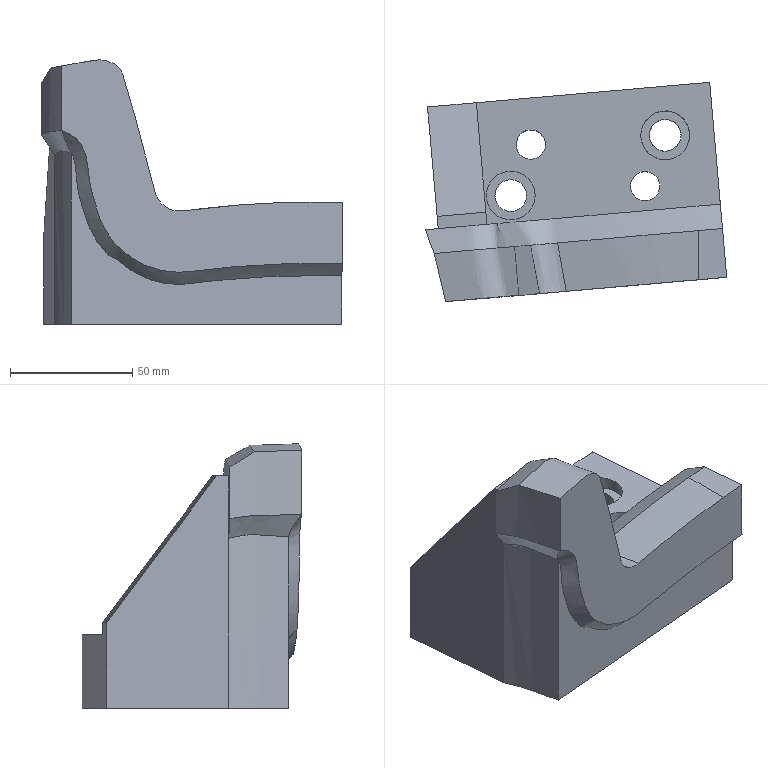Part | NX | features solid 2 | 1 solid | 29 faces | box 123.21 x 89.747 x 108.114 mm | volume 393451 mm3 | plane 13 | spline 10 | cylinder 6 | commonest cylinder face diameters 12 x2 13 x2 20 x2